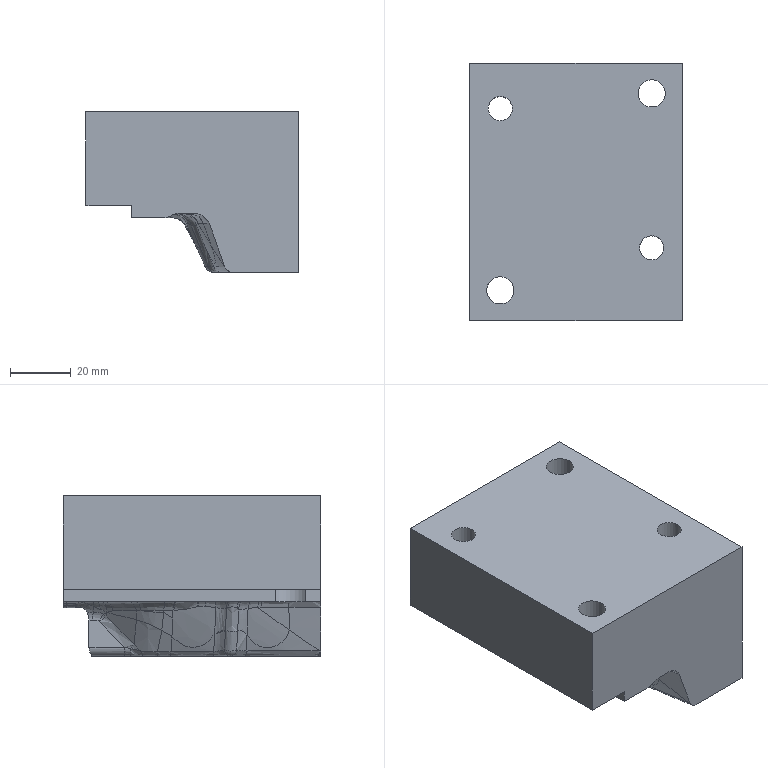Part | STEP file | PN_0037_id1074_x_t | 1 solid | 119 faces | box 70 x 85 x 53 mm | volume 208410 mm3 | spline 75 | plane 26 | cylinder 16 | sphere 2 | commonest cylinder face diameters 10 x8 8 x2 9 x2 14 x2 2 x1 6 x1